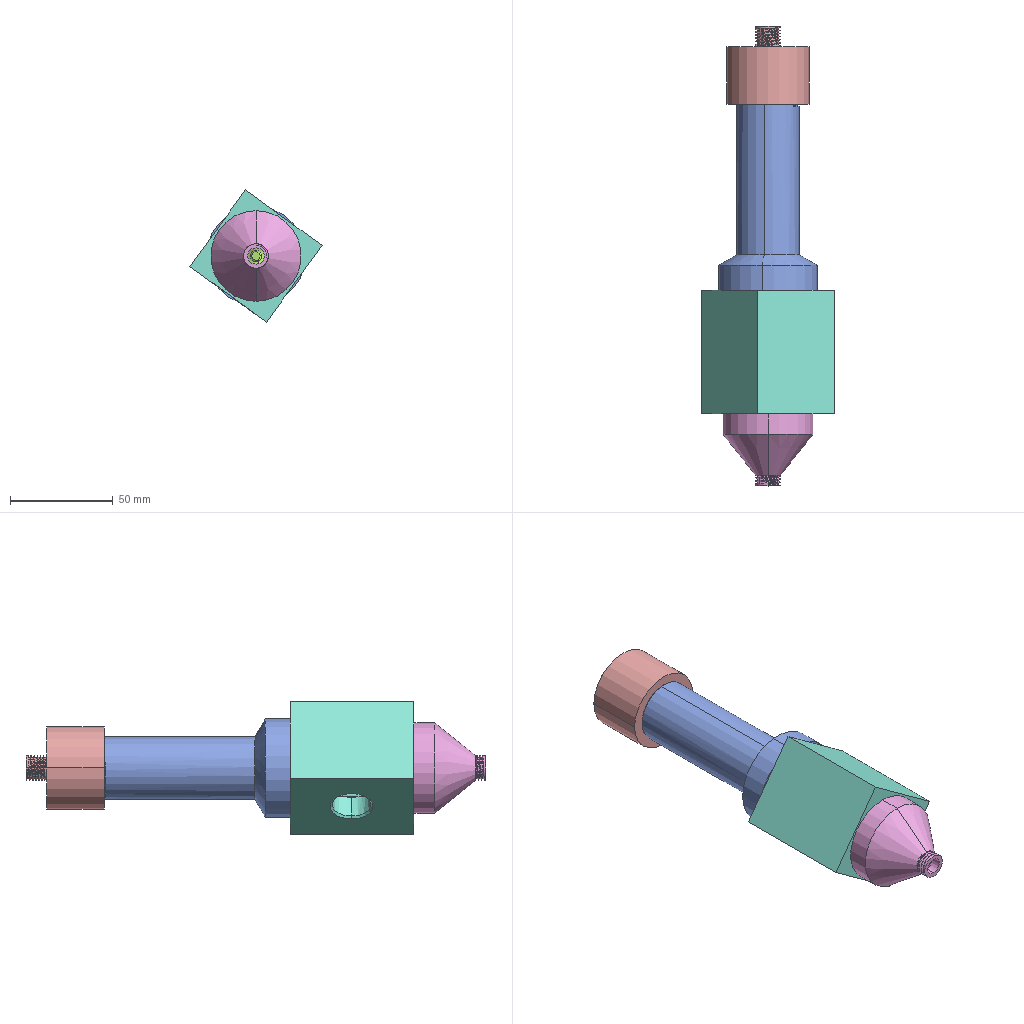Assembly | SolidWorks | 5 different items | 5 placed | box 64 x 223 x 64 mm
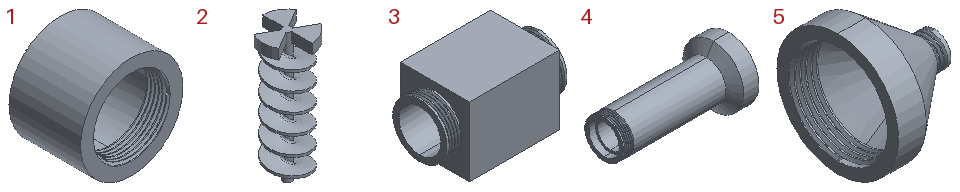Parts list (item | quantity | size | volume | features):
1 | x1 | 40 x 38 x 40 mm | 19573 mm3 | features ICE 4, SweepThread 2, 3DProfileFeature 1, HoleWzd 1, Revolution 1
2 | x1 | 22.43 x 24 x 64 mm | 4107 mm3 | features ICE 2, Extrusion 1, Fillet 1, Helix 1, Sweep 1
3 | x1 | 80 x 46 x 46 mm | 94053 mm3 | features ICE 2, SweepThread 2, 3DProfileFeature 1, Extrusion 1, HoleWzd 1, RefPoint 1
4 | x1 | 98.457 x 48 x 48 mm | 45862 mm3 | features ICE 2, SweepThread 2, Revolution 1
5 | x1 | 35 x 44 x 44 mm | 10879 mm3 | features SweepThread 2, ICE 1, Revolution 1
Mates (type | each side: item.copy, entity, surface, feature):
Concentric | 4.1 edge | 2.1 edge
Coincident | 4.1 face plane Cut-Extrude1 | 2.1 face plane Boss-Extrude2
Concentric | 1.1 edge | 4.1 edge
DistanceDim | 1.1 face plane Boss-Extrude3 | 4.1 face plane Revolve1
Concentric | 4.1 edge | 3.1 edge
Coincident | 4.1 face plane Revolve1 | 3.1 face plane Boss-Extrude1
Concentric | 5.1 edge | 3.1 edge
Coincident | 5.1 face plane Boss-Extrude5 | 3.1 face plane Boss-Extrude1